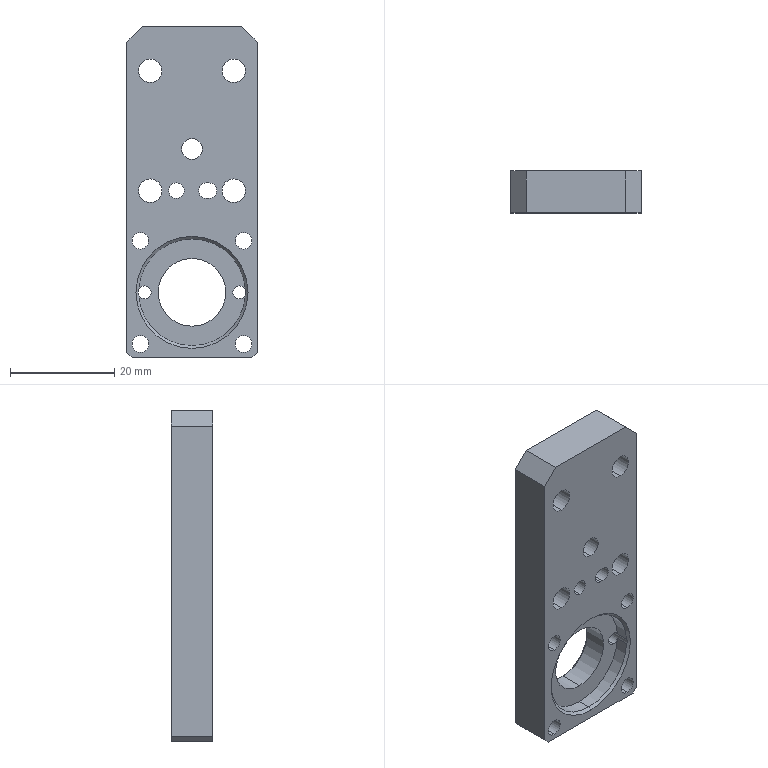Part | SolidWorks | features ICE 6, Chamfer 3, HoleWzd 3, Cut 2, CirPattern 1, Extrusion 1 | 1 solid | 48 faces | box 25 x 8 x 63.5 mm | volume 9911 mm3 | cylinder 31 | plane 13 | cone 4 | commonest cylinder face diameters 3.2 x8 4.5 x8 2.5 x4 3 x4 20.5 x3 4 x2